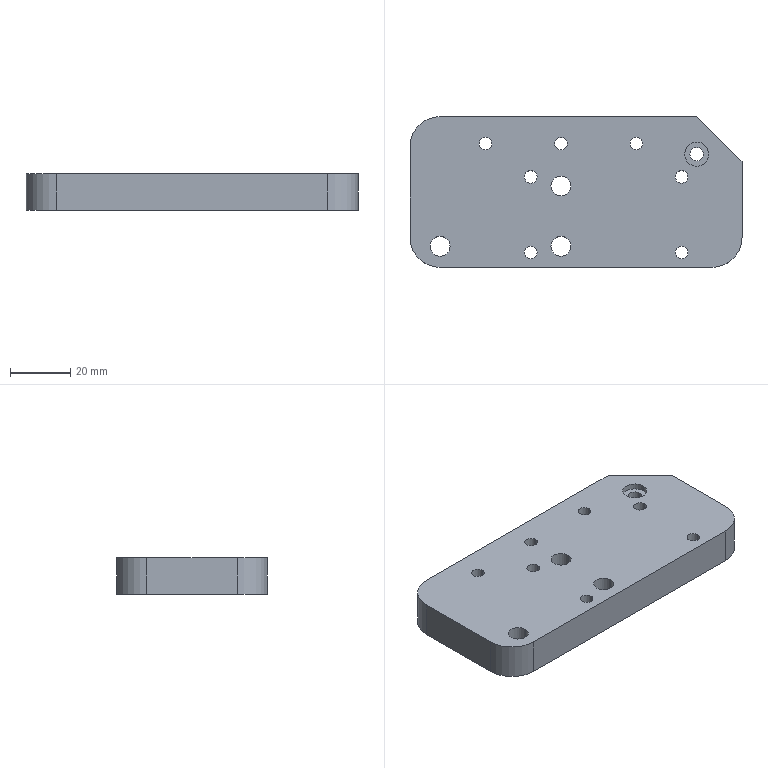Part | STEP file | MT-COMBO-119-S032 | 1 solid | 47 faces | box 110 x 50 x 12 mm | volume 59904 mm3 | cylinder 35 | plane 12 | commonest cylinder face diameters 4.2 x14 6.6 x6 11 x6 8 x4 20 x3 4.5 x2
STEP:
#1=CARTESIAN_POINT('',(-54.5,-43.,6.4));
#2=VERTEX_POINT('',#1);
#3=CARTESIAN_POINT('',(-65.5,-43.,6.4));
#4=VERTEX_POINT('',#3);
#5=CARTESIAN_POINT('',(-60.,-43.,6.4));
#6=DIRECTION('',(0.,0.,-1.));
#7=DIRECTION('',(-1.,0.,0.));
#8=AXIS2_PLACEMENT_3D('',#5,#6,#7);
#9=CIRCLE('',#8,5.5);
#10=EDGE_CURVE('',#2,#4,#9,.T.);
#11=ORIENTED_EDGE('',*,*,#10,.F.);
#12=CARTESIAN_POINT('',(-54.5,-43.,0.));
#13=VERTEX_POINT('',#12);
#14=CARTESIAN_POINT('',(-54.5,-43.,0.));
#15=DIRECTION('',(0.,0.,-1.));
#16=VECTOR('',#15,1000.);
#17=LINE('',#14,#16);
#18=EDGE_CURVE('',#2,#13,#17,.T.);
#19=ORIENTED_EDGE('',*,*,#18,.T.);
#20=CARTESIAN_POINT('',(-65.5,-43.,0.));
#21=VERTEX_POINT('',#20);
#22=CARTESIAN_POINT('',(-60.,-43.,0.));
#23=DIRECTION('',(0.,0.,-1.));
#24=DIRECTION('',(-1.,0.,0.));
#25=AXIS2_PLACEMENT_3D('',#22,#23,#24);
#26=CIRCLE('',#25,5.5);
#27=EDGE_CURVE('',#13,#21,#26,.T.);
#28=ORIENTED_EDGE('',*,*,#27,.T.);
#29=CARTESIAN_POINT('',(-65.5,-43.,0.));
#30=DIRECTION('',(0.,0.,-1.));
#31=VECTOR('',#30,1000.);
#32=LINE('',#29,#31);
#33=EDGE_CURVE('',#4,#21,#32,.T.);
#34=ORIENTED_EDGE('',*,*,#33,.F.);
#35=EDGE_LOOP('',(#11,#19,#28,#34));
#36=FACE_OUTER_BOUND('',#35,.T.);
#37=CARTESIAN_POINT('',(-60.,-43.,0.));
#38=DIRECTION('',(0.,0.,-1.));
#39=DIRECTION('',(-1.,0.,0.));
#40=AXIS2_PLACEMENT_3D('',#37,#38,#39);
#41=CYLINDRICAL_SURFACE('',#40,5.5);
#42=ADVANCED_FACE('',(#36),#41,.F.);
#43=CARTESIAN_POINT('',(-56.7,-43.,12.));
#44=VERTEX_POINT('',#43);
#45=CARTESIAN_POINT('',(-63.3,-43.,12.));
#46=VERTEX_POINT('',#45);
#47=CARTESIAN_POINT('',(-60.,-43.,12.));
#48=DIRECTION('',(0.,0.,-1.));
#49=DIRECTION('',(-1.,0.,0.));
#50=AXIS2_PLACEMENT_3D('',#47,#48,#49);
#51=CIRCLE('',#50,3.3);
#52=EDGE_CURVE('',#44,#46,#51,.T.);
#53=ORIENTED_EDGE('',*,*,#52,.F.);
#54=CARTESIAN_POINT('',(-56.7,-43.,6.4));
#55=VERTEX_POINT('',#54);
#56=CARTESIAN_POINT('',(-56.7,-43.,0.));
#57=DIRECTION('',(0.,0.,-1.));
#58=VECTOR('',#57,1000.);
#59=LINE('',#56,#58);
#60=EDGE_CURVE('',#44,#55,#59,.T.);
#61=ORIENTED_EDGE('',*,*,#60,.T.);
#62=CARTESIAN_POINT('',(-63.3,-43.,6.4));
#63=VERTEX_POINT('',#62);
#64=CARTESIAN_POINT('',(-60.,-43.,6.4));
#65=DIRECTION('',(0.,0.,-1.));
#66=DIRECTION('',(-1.,0.,0.));
#67=AXIS2_PLACEMENT_3D('',#64,#65,#66);
#68=CIRCLE('',#67,3.3);
#69=EDGE_CURVE('',#55,#63,#68,.T.);
#70=ORIENTED_EDGE('',*,*,#69,.T.);
#71=CARTESIAN_POINT('',(-63.3,-43.,0.));
#72=DIRECTION('',(0.,0.,-1.));
#73=VECTOR('',#72,1000.);
#74=LINE('',#71,#73);
#75=EDGE_CURVE('',#46,#63,#74,.T.);
#76=ORIENTED_EDGE('',*,*,#75,.F.);
#77=EDGE_LOOP('',(#53,#61,#70,#76));
#78=FACE_OUTER_BOUND('',#77,.T.);
#79=CARTESIAN_POINT('',(-60.,-43.,0.));
#80=DIRECTION('',(0.,0.,-1.));
#81=DIRECTION('',(-1.,0.,0.));
#82=AXIS2_PLACEMENT_3D('',#79,#80,#81);
#83=CYLINDRICAL_SURFACE('',#82,3.3);
#84=ADVANCED_FACE('',(#78),#83,.F.);
#85=CARTESIAN_POINT('',(-94.5,-43.,6.4));
#86=VERTEX_POINT('',#85);
#87=CARTESIAN_POINT('',(-105.5,-43.,6.4));
#88=VERTEX_POINT('',#87);
#89=CARTESIAN_POINT('',(-100.,-43.,6.4));
#90=DIRECTION('',(0.,0.,-1.));
#91=DIRECTION('',(-1.,0.,0.));
#92=AXIS2_PLACEMENT_3D('',#89,#90,#91);
#93=CIRCLE('',#92,5.5);
#94=EDGE_CURVE('',#86,#88,#93,.T.);
#95=ORIENTED_EDGE('',*,*,#94,.F.);
#96=CARTESIAN_POINT('',(-94.5,-43.,0.));
#97=VERTEX_POINT('',#96);
#98=CARTESIAN_POINT('',(-94.5,-43.,0.));
#99=DIRECTION('',(0.,0.,-1.));
#100=VECTOR('',#99,1000.);
#101=LINE('',#98,#100);
#102=EDGE_CURVE('',#86,#97,#101,.T.);
#103=ORIENTED_EDGE('',*,*,#102,.T.);
#104=CARTESIAN_POINT('',(-105.5,-43.,0.));
#105=VERTEX_POINT('',#104);
#106=CARTESIAN_POINT('',(-100.,-43.,0.));
#107=DIRECTION('',(0.,0.,-1.));
#108=DIRECTION('',(-1.,0.,0.));
#109=AXIS2_PLACEMENT_3D('',#106,#107,#108);
#110=CIRCLE('',#109,5.5);
#111=EDGE_CURVE('',#97,#105,#110,.T.);
#112=ORIENTED_EDGE('',*,*,#111,.T.);
#113=CARTESIAN_POINT('',(-105.5,-43.,0.));
#114=DIRECTION('',(0.,0.,-1.));
#115=VECTOR('',#114,1000.);
#116=LINE('',#113,#115);
#117=EDGE_CURVE('',#88,#105,#116,.T.);
#118=ORIENTED_EDGE('',*,*,#117,.F.);
#119=EDGE_LOOP('',(#95,#103,#112,#118));
#120=FACE_OUTER_BOUND('',#119,.T.);
#121=CARTESIAN_POINT('',(-100.,-43.,0.));
#122=DIRECTION('',(0.,0.,-1.));
#123=DIRECTION('',(-1.,0.,0.));
#124=AXIS2_PLACEMENT_3D('',#121,#122,#123);
#125=CYLINDRICAL_SURFACE('',#124,5.5);
#126=ADVANCED_FACE('',(#120),#125,.F.);
#127=CARTESIAN_POINT('',(-96.7,-43.,12.));
#128=VERTEX_POINT('',#127);
#129=CARTESIAN_POINT('',(-103.3,-43.,12.));
#130=VERTEX_POINT('',#129);
#131=CARTESIAN_POINT('',(-100.,-43.,12.));
#132=DIRECTION('',(0.,0.,-1.));
#133=DIRECTION('',(-1.,0.,0.));
#134=AXIS2_PLACEMENT_3D('',#131,#132,#133);
#135=CIRCLE('',#134,3.3);
#136=EDGE_CURVE('',#128,#130,#135,.T.);
#137=ORIENTED_EDGE('',*,*,#136,.F.);
#138=CARTESIAN_POINT('',(-96.7,-43.,6.4));
#139=VERTEX_POINT('',#138);
#140=CARTESIAN_POINT('',(-96.7,-43.,0.));
#141=DIRECTION('',(0.,0.,-1.));
#142=VECTOR('',#141,1000.);
#143=LINE('',#140,#142);
#144=EDGE_CURVE('',#128,#139,#143,.T.);
#145=ORIENTED_EDGE('',*,*,#144,.T.);
#146=CARTESIAN_POINT('',(-103.3,-43.,6.4));
#147=VERTEX_POINT('',#146);
#148=CARTESIAN_POINT('',(-100.,-43.,6.4));
#149=DIRECTION('',(0.,0.,-1.));
#150=DIRECTION('',(-1.,0.,0.));
#151=AXIS2_PLACEMENT_3D('',#148,#149,#150);
#152=CIRCLE('',#151,3.3);
#153=EDGE_CURVE('',#139,#147,#152,.T.);
#154=ORIENTED_EDGE('',*,*,#153,.T.);
#155=CARTESIAN_POINT('',(-103.3,-43.,0.));
#156=DIRECTION('',(0.,0.,-1.));
#157=VECTOR('',#156,1000.);
#158=LINE('',#155,#157);
#159=EDGE_CURVE('',#130,#147,#158,.T.);
#160=ORIENTED_EDGE('',*,*,#159,.F.);
#161=EDGE_LOOP('',(#137,#145,#154,#160));
#162=FACE_OUTER_BOUND('',#161,.T.);
#163=CARTESIAN_POINT('',(-100.,-43.,0.));
#164=DIRECTION('',(0.,0.,-1.));
#165=DIRECTION('',(-1.,0.,0.));
#166=AXIS2_PLACEMENT_3D('',#163,#164,#165);
#167=CYLINDRICAL_SURFACE('',#166,3.3);
#168=ADVANCED_FACE('',(#162),#167,.F.);
#169=CARTESIAN_POINT('',(-54.5,-23.,6.4));
#170=VERTEX_POINT('',#169);
#171=CARTESIAN_POINT('',(-65.5,-23.,6.4));
#172=VERTEX_POINT('',#171);
#173=CARTESIAN_POINT('',(-60.,-23.,6.4));
#174=DIRECTION('',(0.,0.,-1.));
#175=DIRECTION('',(-1.,0.,0.));
#176=AXIS2_PLACEMENT_3D('',#173,#174,#175);
#177=CIRCLE('',#176,5.5);
#178=EDGE_CURVE('',#170,#172,#177,.T.);
#179=ORIENTED_EDGE('',*,*,#178,.F.);
#180=CARTESIAN_POINT('',(-54.5,-23.,0.));
#181=VERTEX_POINT('',#180);
#182=CARTESIAN_POINT('',(-54.5,-23.,0.));
#183=DIRECTION('',(0.,0.,-1.));
#184=VECTOR('',#183,1000.);
#185=LINE('',#182,#184);
#186=EDGE_CURVE('',#170,#181,#185,.T.);
#187=ORIENTED_EDGE('',*,*,#186,.T.);
#188=CARTESIAN_POINT('',(-65.5,-23.,0.));
#189=VERTEX_POINT('',#188);
#190=CARTESIAN_POINT('',(-60.,-23.,0.));
#191=DIRECTION('',(0.,0.,-1.));
#192=DIRECTION('',(-1.,0.,0.));
#193=AXIS2_PLACEMENT_3D('',#190,#191,#192);
#194=CIRCLE('',#193,5.5);
#195=EDGE_CURVE('',#181,#189,#194,.T.);
#196=ORIENTED_EDGE('',*,*,#195,.T.);
#197=CARTESIAN_POINT('',(-65.5,-23.,0.));
#198=DIRECTION('',(0.,0.,-1.));
#199=VECTOR('',#198,1000.);
#200=LINE('',#197,#199);
#201=EDGE_CURVE('',#172,#189,#200,.T.);
#202=ORIENTED_EDGE('',*,*,#201,.F.);
#203=EDGE_LOOP('',(#179,#187,#196,#202));
#204=FACE_OUTER_BOUND('',#203,.T.);
#205=CARTESIAN_POINT('',(-60.,-23.,0.));
#206=DIRECTION('',(0.,0.,-1.));
#207=DIRECTION('',(-1.,0.,0.));
#208=AXIS2_PLACEMENT_3D('',#205,#206,#207);
#209=CYLINDRICAL_SURFACE('',#208,5.5);
#210=ADVANCED_FACE('',(#204),#209,.F.);
#211=CARTESIAN_POINT('',(-56.7,-23.,12.));
#212=VERTEX_POINT('',#211);
#213=CARTESIAN_POINT('',(-63.3,-23.,12.));
#214=VERTEX_POINT('',#213);
#215=CARTESIAN_POINT('',(-60.,-23.,12.));
#216=DIRECTION('',(0.,0.,-1.));
#217=DIRECTION('',(-1.,0.,0.));
#218=AXIS2_PLACEMENT_3D('',#215,#216,#217);
#219=CIRCLE('',#218,3.3);
#220=EDGE_CURVE('',#212,#214,#219,.T.);
#221=ORIENTED_EDGE('',*,*,#220,.F.);
#222=CARTESIAN_POINT('',(-56.7,-23.,6.4));
#223=VERTEX_POINT('',#222);
#224=CARTESIAN_POINT('',(-56.7,-23.,0.));
#225=DIRECTION('',(0.,0.,-1.));
#226=VECTOR('',#225,1000.);
#227=LINE('',#224,#226);
#228=EDGE_CURVE('',#212,#223,#227,.T.);
#229=ORIENTED_EDGE('',*,*,#228,.T.);
#230=CARTESIAN_POINT('',(-63.3,-23.,6.4));
#231=VERTEX_POINT('',#230);
#232=CARTESIAN_POINT('',(-60.,-23.,6.4));
#233=DIRECTION('',(0.,0.,-1.));
#234=DIRECTION('',(-1.,0.,0.));
#235=AXIS2_PLACEMENT_3D('',#232,#233,#234);
#236=CIRCLE('',#235,3.3);
#237=EDGE_CURVE('',#223,#231,#236,.T.);
#238=ORIENTED_EDGE('',*,*,#237,.T.);
#239=CARTESIAN_POINT('',(-63.3,-23.,0.));
#240=DIRECTION('',(0.,0.,-1.));
#241=VECTOR('',#240,1000.);
#242=LINE('',#239,#241);
#243=EDGE_CURVE('',#214,#231,#242,.T.);
#244=ORIENTED_EDGE('',*,*,#243,.F.);
#245=EDGE_LOOP('',(#221,#229,#238,#244));
#246=FACE_OUTER_BOUND('',#245,.T.);
#247=CARTESIAN_POINT('',(-60.,-23.,0.));
#248=DIRECTION('',(0.,0.,-1.));
#249=DIRECTION('',(-1.,0.,0.));
#250=AXIS2_PLACEMENT_3D('',#247,#248,#249);
#251=CYLINDRICAL_SURFACE('',#250,3.3);
#252=ADVANCED_FACE('',(#246),#251,.F.);
#253=CARTESIAN_POINT('',(-32.9,-9.,12.));
#254=VERTEX_POINT('',#253);
#255=CARTESIAN_POINT('',(-37.1,-9.,12.));
#256=VERTEX_POINT('',#255);
#257=CARTESIAN_POINT('',(-35.,-9.,12.));
#258=DIRECTION('',(0.,0.,-1.));
#259=DIRECTION('',(-1.,0.,0.));
#260=AXIS2_PLACEMENT_3D('',#257,#258,#259);
#261=CIRCLE('',#260,2.1);
#262=EDGE_CURVE('',#254,#256,#261,.T.);
#263=ORIENTED_EDGE('',*,*,#262,.F.);
#264=CARTESIAN_POINT('',(-32.9,-9.,0.));
#265=VERTEX_POINT('',#264);
#266=CARTESIAN_POINT('',(-32.9,-9.,0.));
#267=DIRECTION('',(0.,0.,-1.));
#268=VECTOR('',#267,1000.);
#269=LINE('',#266,#268);
#270=EDGE_CURVE('',#254,#265,#269,.T.);
#271=ORIENTED_EDGE('',*,*,#270,.T.);
#272=CARTESIAN_POINT('',(-37.1,-9.,0.));
#273=VERTEX_POINT('',#272);
#274=CARTESIAN_POINT('',(-35.,-9.,0.));
#275=DIRECTION('',(0.,0.,-1.));
#276=DIRECTION('',(-1.,0.,0.));
#277=AXIS2_PLACEMENT_3D('',#274,#275,#276);
#278=CIRCLE('',#277,2.1);
#279=EDGE_CURVE('',#265,#273,#278,.T.);
#280=ORIENTED_EDGE('',*,*,#279,.T.);
#281=CARTESIAN_POINT('',(-37.1,-9.,0.));
#282=DIRECTION('',(0.,0.,-1.));
#283=VECTOR('',#282,1000.);
#284=LINE('',#281,#283);
#285=EDGE_CURVE('',#256,#273,#284,.T.);
#286=ORIENTED_EDGE('',*,*,#285,.F.);
#287=EDGE_LOOP('',(#263,#271,#280,#286));
#288=FACE_OUTER_BOUND('',#287,.T.);
#289=CARTESIAN_POINT('',(-35.,-9.,0.));
#290=DIRECTION('',(0.,0.,-1.));
#291=DIRECTION('',(-1.,0.,0.));
#292=AXIS2_PLACEMENT_3D('',#289,#290,#291);
#293=CYLINDRICAL_SURFACE('',#292,2.1);
#294=ADVANCED_FACE('',(#288),#293,.F.);
#295=CARTESIAN_POINT('',(-57.9,-9.,12.));
#296=VERTEX_POINT('',#295);
#297=CARTESIAN_POINT('',(-62.1,-9.,12.));
#298=VERTEX_POINT('',#297);
#299=CARTESIAN_POINT('',(-60.,-9.,12.));
#300=DIRECTION('',(0.,0.,-1.));
#301=DIRECTION('',(-1.,0.,0.));
#302=AXIS2_PLACEMENT_3D('',#299,#300,#301);
#303=CIRCLE('',#302,2.1);
#304=EDGE_CURVE('',#296,#298,#303,.T.);
#305=ORIENTED_EDGE('',*,*,#304,.F.);
#306=CARTESIAN_POINT('',(-57.9,-9.,0.));
#307=VERTEX_POINT('',#306);
#308=CARTESIAN_POINT('',(-57.9,-9.,0.));
#309=DIRECTION('',(0.,0.,-1.));
#310=VECTOR('',#309,1000.);
#311=LINE('',#308,#310);
#312=EDGE_CURVE('',#296,#307,#311,.T.);
#313=ORIENTED_EDGE('',*,*,#312,.T.);
#314=CARTESIAN_POINT('',(-62.1,-9.,0.));
#315=VERTEX_POINT('',#314);
#316=CARTESIAN_POINT('',(-60.,-9.,0.));
#317=DIRECTION('',(0.,0.,-1.));
#318=DIRECTION('',(-1.,0.,0.));
#319=AXIS2_PLACEMENT_3D('',#316,#317,#318);
#320=CIRCLE('',#319,2.1);
#321=EDGE_CURVE('',#307,#315,#320,.T.);
#322=ORIENTED_EDGE('',*,*,#321,.T.);
#323=CARTESIAN_POINT('',(-62.1,-9.,0.));
#324=DIRECTION('',(0.,0.,-1.));
#325=VECTOR('',#324,1000.);
#326=LINE('',#323,#325);
#327=EDGE_CURVE('',#298,#315,#326,.T.);
#328=ORIENTED_EDGE('',*,*,#327,.F.);
#329=EDGE_LOOP('',(#305,#313,#322,#328));
#330=FACE_OUTER_BOUND('',#329,.T.);
#331=CARTESIAN_POINT('',(-60.,-9.,0.));
#332=DIRECTION('',(0.,0.,-1.));
#333=DIRECTION('',(-1.,0.,0.));
#334=AXIS2_PLACEMENT_3D('',#331,#332,#333);
#335=CYLINDRICAL_SURFACE('',#334,2.1);
#336=ADVANCED_FACE('',(#330),#335,.F.);
#337=CARTESIAN_POINT('',(-82.9,-9.,12.));
#338=VERTEX_POINT('',#337);
#339=CARTESIAN_POINT('',(-87.1,-9.,12.));
#340=VERTEX_POINT('',#339);
#341=CARTESIAN_POINT('',(-85.,-9.,12.));
#342=DIRECTION('',(0.,0.,-1.));
#343=DIRECTION('',(-1.,0.,0.));
#344=AXIS2_PLACEMENT_3D('',#341,#342,#343);
#345=CIRCLE('',#344,2.1);
#346=EDGE_CURVE('',#338,#340,#345,.T.);
#347=ORIENTED_EDGE('',*,*,#346,.F.);
#348=CARTESIAN_POINT('',(-82.9,-9.,0.));
#349=VERTEX_POINT('',#348);
#350=CARTESIAN_POINT('',(-82.9,-9.,0.));
#351=DIRECTION('',(0.,0.,-1.));
#352=VECTOR('',#351,1000.);
#353=LINE('',#350,#352);
#354=EDGE_CURVE('',#338,#349,#353,.T.);
#355=ORIENTED_EDGE('',*,*,#354,.T.);
#356=CARTESIAN_POINT('',(-87.1,-9.,0.));
#357=VERTEX_POINT('',#356);
#358=CARTESIAN_POINT('',(-85.,-9.,0.));
#359=DIRECTION('',(0.,0.,-1.));
#360=DIRECTION('',(-1.,0.,0.));
#361=AXIS2_PLACEMENT_3D('',#358,#359,#360);
#362=CIRCLE('',#361,2.1);
#363=EDGE_CURVE('',#349,#357,#362,.T.);
#364=ORIENTED_EDGE('',*,*,#363,.T.);
#365=CARTESIAN_POINT('',(-87.1,-9.,0.));
#366=DIRECTION('',(0.,0.,-1.));
#367=VECTOR('',#366,1000.);
#368=LINE('',#365,#367);
#369=EDGE_CURVE('',#340,#357,#368,.T.);
#370=ORIENTED_EDGE('',*,*,#369,.F.);
#371=EDGE_LOOP('',(#347,#355,#364,#370));
#372=FACE_OUTER_BOUND('',#371,.T.);
#373=CARTESIAN_POINT('',(-85.,-9.,0.));
#374=DIRECTION('',(0.,0.,-1.));
#375=DIRECTION('',(-1.,0.,0.));
#376=AXIS2_PLACEMENT_3D('',#373,#374,#375);
#377=CYLINDRICAL_SURFACE('',#376,2.1);
#378=ADVANCED_FACE('',(#372),#377,.F.);
#379=CARTESIAN_POINT('',(-67.9,-20.,12.));
#380=VERTEX_POINT('',#379);
#381=CARTESIAN_POINT('',(-72.1,-20.,12.));
#382=VERTEX_POINT('',#381);
#383=CARTESIAN_POINT('',(-70.,-20.,12.));
#384=DIRECTION('',(0.,0.,-1.));
#385=DIRECTION('',(-1.,0.,0.));
#386=AXIS2_PLACEMENT_3D('',#383,#384,#385);
#387=CIRCLE('',#386,2.1);
#388=EDGE_CURVE('',#380,#382,#387,.T.);
#389=ORIENTED_EDGE('',*,*,#388,.F.);
#390=CARTESIAN_POINT('',(-67.9,-20.,0.));
#391=VERTEX_POINT('',#390);
#392=CARTESIAN_POINT('',(-67.9,-20.,0.));
#393=DIRECTION('',(0.,0.,-1.));
#394=VECTOR('',#393,1000.);
#395=LINE('',#392,#394);
#396=EDGE_CURVE('',#380,#391,#395,.T.);
#397=ORIENTED_EDGE('',*,*,#396,.T.);
#398=CARTESIAN_POINT('',(-72.1,-20.,0.));
#399=VERTEX_POINT('',#398);
#400=CARTESIAN_POINT('',(-70.,-20.,0.));
#401=DIRECTION('',(0.,0.,-1.));
#402=DIRECTION('',(-1.,0.,0.));
#403=AXIS2_PLACEMENT_3D('',#400,#401,#402);
#404=CIRCLE('',#403,2.1);
#405=EDGE_CURVE('',#391,#399,#404,.T.);
#406=ORIENTED_EDGE('',*,*,#405,.T.);
#407=CARTESIAN_POINT('',(-72.1,-20.,0.));
#408=DIRECTION('',(0.,0.,-1.));
#409=VECTOR('',#408,1000.);
#410=LINE('',#407,#409);
#411=EDGE_CURVE('',#382,#399,#410,.T.);
#412=ORIENTED_EDGE('',*,*,#411,.F.);
#413=EDGE_LOOP('',(#389,#397,#406,#412));
#414=FACE_OUTER_BOUND('',#413,.T.);
#415=CARTESIAN_POINT('',(-70.,-20.,0.));
#416=DIRECTION('',(0.,0.,-1.));
#417=DIRECTION('',(-1.,0.,0.));
#418=AXIS2_PLACEMENT_3D('',#415,#416,#417);
#419=CYLINDRICAL_SURFACE('',#418,2.1);
#420=ADVANCED_FACE('',(#414),#419,.F.);
#421=CARTESIAN_POINT('',(-67.9,-45.,12.));
#422=VERTEX_POINT('',#421);
#423=CARTESIAN_POINT('',(-72.1,-45.,12.));
#424=VERTEX_POINT('',#423);
#425=CARTESIAN_POINT('',(-70.,-45.,12.));
#426=DIRECTION('',(0.,0.,-1.));
#427=DIRECTION('',(-1.,0.,0.));
#428=AXIS2_PLACEMENT_3D('',#425,#426,#427);
#429=CIRCLE('',#428,2.1);
#430=EDGE_CURVE('',#422,#424,#429,.T.);
#431=ORIENTED_EDGE('',*,*,#430,.F.);
#432=CARTESIAN_POINT('',(-67.9,-45.,0.));
#433=VERTEX_POINT('',#432);
#434=CARTESIAN_POINT('',(-67.9,-45.,0.));
#435=DIRECTION('',(0.,0.,-1.));
#436=VECTOR('',#435,1000.);
#437=LINE('',#434,#436);
#438=EDGE_CURVE('',#422,#433,#437,.T.);
#439=ORIENTED_EDGE('',*,*,#438,.T.);
#440=CARTESIAN_POINT('',(-72.1,-45.,0.));
#441=VERTEX_POINT('',#440);
#442=CARTESIAN_POINT('',(-70.,-45.,0.));
#443=DIRECTION('',(0.,0.,-1.));
#444=DIRECTION('',(-1.,0.,0.));
#445=AXIS2_PLACEMENT_3D('',#442,#443,#444);
#446=CIRCLE('',#445,2.1);
#447=EDGE_CURVE('',#433,#441,#446,.T.);
#448=ORIENTED_EDGE('',*,*,#447,.T.);
#449=CARTESIAN_POINT('',(-72.1,-45.,0.));
#450=DIRECTION('',(0.,0.,-1.));
#451=VECTOR('',#450,1000.);
#452=LINE('',#449,#451);
#453=EDGE_CURVE('',#424,#441,#452,.T.);
#454=ORIENTED_EDGE('',*,*,#453,.F.);
#455=EDGE_LOOP('',(#431,#439,#448,#454));
#456=FACE_OUTER_BOUND('',#455,.T.);
#457=CARTESIAN_POINT('',(-70.,-45.,0.));
#458=DIRECTION('',(0.,0.,-1.));
#459=DIRECTION('',(-1.,0.,0.));
#460=AXIS2_PLACEMENT_3D('',#457,#458,#459);
#461=CYLINDRICAL_SURFACE('',#460,2.1);
#462=ADVANCED_FACE('',(#456),#461,.F.);
#463=CARTESIAN_POINT('',(-17.9,-45.,12.));
#464=VERTEX_POINT('',#463);
#465=CARTESIAN_POINT('',(-22.1,-45.,12.));
#466=VERTEX_POINT('',#465);
#467=CARTESIAN_POINT('',(-20.,-45.,12.));
#468=DIRECTION('',(0.,0.,-1.));
#469=DIRECTION('',(-1.,0.,0.));
#470=AXIS2_PLACEMENT_3D('',#467,#468,#469);
#471=CIRCLE('',#470,2.1);
#472=EDGE_CURVE('',#464,#466,#471,.T.);
#473=ORIENTED_EDGE('',*,*,#472,.F.);
#474=CARTESIAN_POINT('',(-17.9,-45.,0.));
#475=VERTEX_POINT('',#474);
#476=CARTESIAN_POINT('',(-17.9,-45.,0.));
#477=DIRECTION('',(0.,0.,-1.));
#478=VECTOR('',#477,1000.);
#479=LINE('',#476,#478);
#480=EDGE_CURVE('',#464,#475,#479,.T.);
#481=ORIENTED_EDGE('',*,*,#480,.T.);
#482=CARTESIAN_POINT('',(-22.1,-45.,0.));
#483=VERTEX_POINT('',#482);
#484=CARTESIAN_POINT('',(-20.,-45.,0.));
#485=DIRECTION('',(0.,0.,-1.));
#486=DIRECTION('',(-1.,0.,0.));
#487=AXIS2_PLACEMENT_3D('',#484,#485,#486);
#488=CIRCLE('',#487,2.1);
#489=EDGE_CURVE('',#475,#483,#488,.T.);
#490=ORIENTED_EDGE('',*,*,#489,.T.);
#491=CARTESIAN_POINT('',(-22.1,-45.,0.));
#492=DIRECTION('',(0.,0.,-1.));
#493=VECTOR('',#492,1000.);
#494=LINE('',#491,#493);
#495=EDGE_CURVE('',#466,#483,#494,.T.);
#496=ORIENTED_EDGE('',*,*,#495,.F.);
#497=EDGE_LOOP('',(#473,#481,#490,#496));
#498=FACE_OUTER_BOUND('',#497,.T.);
#499=CARTESIAN_POINT('',(-20.,-45.,0.));
#500=DIRECTION('',(0.,0.,-1.));
#501=DIRECTION('',(-1.,0.,0.));
#502=AXIS2_PLACEMENT_3D('',#499,#500,#501);
#503=CYLINDRICAL_SURFACE('',#502,2.1);
#504=ADVANCED_FACE('',(#498),#503,.F.);
#505=CARTESIAN_POINT('',(-17.9,-20.,12.));
#506=VERTEX_POINT('',#505);
#507=CARTESIAN_POINT('',(-22.1,-20.,12.));
#508=VERTEX_POINT('',#507);
#509=CARTESIAN_POINT('',(-20.,-20.,12.));
#510=DIRECTION('',(0.,0.,-1.));
#511=DIRECTION('',(-1.,0.,0.));
#512=AXIS2_PLACEMENT_3D('',#509,#510,#511);
#513=CIRCLE('',#512,2.1);
#514=EDGE_CURVE('',#506,#508,#513,.T.);
#515=ORIENTED_EDGE('',*,*,#514,.F.);
#516=CARTESIAN_POINT('',(-17.9,-20.,0.));
#517=VERTEX_POINT('',#516);
#518=CARTESIAN_POINT('',(-17.9,-20.,0.));
#519=DIRECTION('',(0.,0.,-1.));
#520=VECTOR('',#519,1000.);
#521=LINE('',#518,#520);
#522=EDGE_CURVE('',#506,#517,#521,.T.);
#523=ORIENTED_EDGE('',*,*,#522,.T.);
#524=CARTESIAN_POINT('',(-22.1,-20.,0.));
#525=VERTEX_POINT('',#524);
#526=CARTESIAN_POINT('',(-20.,-20.,0.));
#527=DIRECTION('',(0.,0.,-1.));
#528=DIRECTION('',(-1.,0.,0.));
#529=AXIS2_PLACEMENT_3D('',#526,#527,#528);
#530=CIRCLE('',#529,2.1);
#531=EDGE_CURVE('',#517,#525,#530,.T.);
#532=ORIENTED_EDGE('',*,*,#531,.T.);
#533=CARTESIAN_POINT('',(-22.1,-20.,0.));
#534=DIRECTION('',(0.,0.,-1.));
#535=VECTOR('',#534,1000.);
#536=LINE('',#533,#535);
#537=EDGE_CURVE('',#508,#525,#536,.T.);
#538=ORIENTED_EDGE('',*,*,#537,.F.);
#539=EDGE_LOOP('',(#515,#523,#532,#538));
#540=FACE_OUTER_BOUND('',#539,.T.);
#541=CARTESIAN_POINT('',(-20.,-20.,0.));
#542=DIRECTION('',(0.,0.,-1.));
#543=DIRECTION('',(-1.,0.,0.));
#544=AXIS2_PLACEMENT_3D('',#541,#542,#543);
#545=CYLINDRICAL_SURFACE('',#544,2.1);
#546=ADVANCED_FACE('',(#540),#545,.F.);
#547=CARTESIAN_POINT('',(-19.,-12.5,10.));
#548=VERTEX_POINT('',#547);
#549=CARTESIAN_POINT('',(-11.,-12.5,10.));
#550=VERTEX_POINT('',#549);
#551=CARTESIAN_POINT('',(-15.,-12.5,10.));
#552=DIRECTION('',(0.,0.,1.));
#553=DIRECTION('',(1.,0.,0.));
#554=AXIS2_PLACEMENT_3D('',#551,#552,#553);
#555=CIRCLE('',#554,4.);
#556=EDGE_CURVE('',#548,#550,#555,.T.);
#557=ORIENTED_EDGE('',*,*,#556,.F.);
#558=CARTESIAN_POINT('',(-19.,-12.5,12.));
#559=VERTEX_POINT('',#558);
#560=CARTESIAN_POINT('',(-19.,-12.5,12.));
#561=DIRECTION('',(0.,0.,1.));
#562=VECTOR('',#561,1000.);
#563=LINE('',#560,#562);
#564=EDGE_CURVE('',#548,#559,#563,.T.);
#565=ORIENTED_EDGE('',*,*,#564,.T.);
#566=CARTESIAN_POINT('',(-11.,-12.5,12.));
#567=VERTEX_POINT('',#566);
#568=CARTESIAN_POINT('',(-15.,-12.5,12.));
#569=DIRECTION('',(0.,0.,1.));
#570=DIRECTION('',(1.,0.,0.));
#571=AXIS2_PLACEMENT_3D('',#568,#569,#570);
#572=CIRCLE('',#571,4.);
#573=EDGE_CURVE('',#559,#567,#572,.T.);
#574=ORIENTED_EDGE('',*,*,#573,.T.);
#575=CARTESIAN_POINT('',(-11.,-12.5,12.));
#576=DIRECTION('',(0.,0.,1.));
#577=VECTOR('',#576,1000.);
#578=LINE('',#575,#577);
#579=EDGE_CURVE('',#550,#567,#578,.T.);
#580=ORIENTED_EDGE('',*,*,#579,.F.);
#581=EDGE_LOOP('',(#557,#565,#574,#580));
#582=FACE_OUTER_BOUND('',#581,.T.);
#583=CARTESIAN_POINT('',(-15.,-12.5,12.));
#584=DIRECTION('',(0.,0.,1.));
#585=DIRECTION('',(1.,0.,0.));
#586=AXIS2_PLACEMENT_3D('',#583,#584,#585);
#587=CYLINDRICAL_SURFACE('',#586,4.);
#588=ADVANCED_FACE('',(#582),#587,.F.);
#589=CARTESIAN_POINT('',(-11.,-12.5,4.4));
#590=VERTEX_POINT('',#589);
#591=CARTESIAN_POINT('',(-19.,-12.5,4.4));
#592=VERTEX_POINT('',#591);
#593=CARTESIAN_POINT('',(-15.,-12.5,4.4));
#594=DIRECTION('',(0.,0.,-1.));
#595=DIRECTION('',(-1.,0.,0.));
#596=AXIS2_PLACEMENT_3D('',#593,#594,#595);
#597=CIRCLE('',#596,4.);
#598=EDGE_CURVE('',#590,#592,#597,.T.);
#599=ORIENTED_EDGE('',*,*,#598,.F.);
#600=CARTESIAN_POINT('',(-11.,-12.5,0.));
#601=VERTEX_POINT('',#600);
#602=CARTESIAN_POINT('',(-11.,-12.5,0.));
#603=DIRECTION('',(0.,0.,-1.));
#604=VECTOR('',#603,1000.);
#605=LINE('',#602,#604);
#606=EDGE_CURVE('',#590,#601,#605,.T.);
#607=ORIENTED_EDGE('',*,*,#606,.T.);
#608=CARTESIAN_POINT('',(-19.,-12.5,0.));
#609=VERTEX_POINT('',#608);
#610=CARTESIAN_POINT('',(-15.,-12.5,0.));
#611=DIRECTION('',(0.,0.,-1.));
#612=DIRECTION('',(-1.,0.,0.));
#613=AXIS2_PLACEMENT_3D('',#610,#611,#612);
#614=CIRCLE('',#613,4.);
#615=EDGE_CURVE('',#601,#609,#614,.T.);
#616=ORIENTED_EDGE('',*,*,#615,.T.);
#617=CARTESIAN_POINT('',(-19.,-12.5,0.));
#618=DIRECTION('',(0.,0.,-1.));
#619=VECTOR('',#618,1000.);
#620=LINE('',#617,#619);
#621=EDGE_CURVE('',#592,#609,#620,.T.);
#622=ORIENTED_EDGE('',*,*,#621,.F.);
#623=EDGE_LOOP('',(#599,#607,#616,#622));
#624=FACE_OUTER_BOUND('',#623,.T.);
#625=CARTESIAN_POINT('',(-15.,-12.5,0.));
#626=DIRECTION('',(0.,0.,-1.));
#627=DIRECTION('',(-1.,0.,0.));
#628=AXIS2_PLACEMENT_3D('',#625,#626,#627);
#629=CYLINDRICAL_SURFACE('',#628,4.);
#630=ADVANCED_FACE('',(#624),#629,.F.);
#631=CARTESIAN_POINT('',(-17.25,-12.5,10.));
#632=VERTEX_POINT('',#631);
#633=CARTESIAN_POINT('',(-12.75,-12.5,10.));
#634=VERTEX_POINT('',#633);
#635=CARTESIAN_POINT('',(-15.,-12.5,10.));
#636=DIRECTION('',(0.,0.,1.));
#637=DIRECTION('',(-1.,0.,0.));
#638=AXIS2_PLACEMENT_3D('',#635,#636,#637);
#639=CIRCLE('',#638,2.25);
#640=EDGE_CURVE('',#632,#634,#639,.T.);
#641=ORIENTED_EDGE('',*,*,#640,.T.);
#642=CARTESIAN_POINT('',(-12.75,-12.5,4.4));
#643=VERTEX_POINT('',#642);
#644=CARTESIAN_POINT('',(-12.75,-12.5,0.));
#645=DIRECTION('',(0.,0.,-1.));
#646=VECTOR('',#645,1000.);
#647=LINE('',#644,#646);
#648=EDGE_CURVE('',#634,#643,#647,.T.);
#649=ORIENTED_EDGE('',*,*,#648,.T.);
#650=CARTESIAN_POINT('',(-17.25,-12.5,4.4));
#651=VERTEX_POINT('',#650);
#652=CARTESIAN_POINT('',(-15.,-12.5,4.4));
#653=DIRECTION('',(0.,0.,-1.));
#654=DIRECTION('',(-1.,0.,0.));
#655=AXIS2_PLACEMENT_3D('',#652,#653,#654);
#656=CIRCLE('',#655,2.25);
#657=EDGE_CURVE('',#643,#651,#656,.T.);
#658=ORIENTED_EDGE('',*,*,#657,.T.);
#659=CARTESIAN_POINT('',(-17.25,-12.5,0.));
#660=DIRECTION('',(0.,0.,-1.));
#661=VECTOR('',#660,1000.);
#662=LINE('',#659,#661);
#663=EDGE_CURVE('',#632,#651,#662,.T.);
#664=ORIENTED_EDGE('',*,*,#663,.F.);
#665=EDGE_LOOP('',(#641,#649,#658,#664));
#666=FACE_OUTER_BOUND('',#665,.T.);
#667=CARTESIAN_POINT('',(-15.,-12.5,0.));
#668=DIRECTION('',(0.,0.,-1.));
#669=DIRECTION('',(-1.,0.,0.));
#670=AXIS2_PLACEMENT_3D('',#667,#668,#669);
#671=CYLINDRICAL_SURFACE('',#670,2.25);
#672=ADVANCED_FACE('',(#666),#671,.F.);
#673=CARTESIAN_POINT('',(-60.,-43.,0.));
#674=DIRECTION('',(0.,0.,-1.));
#675=DIRECTION('',(-1.,0.,0.));
#676=AXIS2_PLACEMENT_3D('',#673,#674,#675);
#677=CIRCLE('',#676,5.5);
#678=EDGE_CURVE('',#21,#13,#677,.T.);
#679=ORIENTED_EDGE('',*,*,#678,.F.);
#680=ORIENTED_EDGE('',*,*,#27,.F.);
#681=EDGE_LOOP('',(#679,#680));
#682=FACE_BOUND('',#681,.T.);
#683=CARTESIAN_POINT('',(-100.,-43.,0.));
#684=DIRECTION('',(0.,0.,-1.));
#685=DIRECTION('',(-1.,0.,0.));
#686=AXIS2_PLACEMENT_3D('',#683,#684,#685);
#687=CIRCLE('',#686,5.5);
#688=EDGE_CURVE('',#105,#97,#687,.T.);
#689=ORIENTED_EDGE('',*,*,#688,.F.);
#690=ORIENTED_EDGE('',*,*,#111,.F.);
#691=EDGE_LOOP('',(#689,#690));
#692=FACE_BOUND('',#691,.T.);
#693=CARTESIAN_POINT('',(-60.,-23.,0.));
#694=DIRECTION('',(0.,0.,-1.));
#695=DIRECTION('',(-1.,0.,0.));
#696=AXIS2_PLACEMENT_3D('',#693,#694,#695);
#697=CIRCLE('',#696,5.5);
#698=EDGE_CURVE('',#189,#181,#697,.T.);
#699=ORIENTED_EDGE('',*,*,#698,.F.);
#700=ORIENTED_EDGE('',*,*,#195,.F.);
#701=EDGE_LOOP('',(#699,#700));
#702=FACE_BOUND('',#701,.T.);
#703=CARTESIAN_POINT('',(-35.,-9.,0.));
#704=DIRECTION('',(0.,0.,-1.));
#705=DIRECTION('',(-1.,0.,0.));
#706=AXIS2_PLACEMENT_3D('',#703,#704,#705);
#707=CIRCLE('',#706,2.1);
#708=EDGE_CURVE('',#273,#265,#707,.T.);
#709=ORIENTED_EDGE('',*,*,#708,.F.);
#710=ORIENTED_EDGE('',*,*,#279,.F.);
#711=EDGE_LOOP('',(#709,#710));
#712=FACE_BOUND('',#711,.T.);
#713=CARTESIAN_POINT('',(-60.,-9.,0.));
#714=DIRECTION('',(0.,0.,-1.));
#715=DIRECTION('',(-1.,0.,0.));
#716=AXIS2_PLACEMENT_3D('',#713,#714,#715);
#717=CIRCLE('',#716,2.1);
#718=EDGE_CURVE('',#315,#307,#717,.T.);
#719=ORIENTED_EDGE('',*,*,#718,.F.);
#720=ORIENTED_EDGE('',*,*,#321,.F.);
#721=EDGE_LOOP('',(#719,#720));
#722=FACE_BOUND('',#721,.T.);
#723=CARTESIAN_POINT('',(-85.,-9.,0.));
#724=DIRECTION('',(0.,0.,-1.));
#725=DIRECTION('',(-1.,0.,0.));
#726=AXIS2_PLACEMENT_3D('',#723,#724,#725);
#727=CIRCLE('',#726,2.1);
#728=EDGE_CURVE('',#357,#349,#727,.T.);
#729=ORIENTED_EDGE('',*,*,#728,.F.);
#730=ORIENTED_EDGE('',*,*,#363,.F.);
#731=EDGE_LOOP('',(#729,#730));
#732=FACE_BOUND('',#731,.T.);
#733=CARTESIAN_POINT('',(-70.,-20.,0.));
#734=DIRECTION('',(0.,0.,-1.));
#735=DIRECTION('',(-1.,0.,0.));
#736=AXIS2_PLACEMENT_3D('',#733,#734,#735);
#737=CIRCLE('',#736,2.1);
#738=EDGE_CURVE('',#399,#391,#737,.T.);
#739=ORIENTED_EDGE('',*,*,#738,.F.);
#740=ORIENTED_EDGE('',*,*,#405,.F.);
#741=EDGE_LOOP('',(#739,#740));
#742=FACE_BOUND('',#741,.T.);
#743=CARTESIAN_POINT('',(-70.,-45.,0.));
#744=DIRECTION('',(0.,0.,-1.));
#745=DIRECTION('',(-1.,0.,0.));
#746=AXIS2_PLACEMENT_3D('',#743,#744,#745);
#747=CIRCLE('',#746,2.1);
#748=EDGE_CURVE('',#441,#433,#747,.T.);
#749=ORIENTED_EDGE('',*,*,#748,.F.);
#750=ORIENTED_EDGE('',*,*,#447,.F.);
#751=EDGE_LOOP('',(#749,#750));
#752=FACE_BOUND('',#751,.T.);
#753=CARTESIAN_POINT('',(-20.,-45.,0.));
#754=DIRECTION('',(0.,0.,-1.));
#755=DIRECTION('',(-1.,0.,0.));
#756=AXIS2_PLACEMENT_3D('',#753,#754,#755);
#757=CIRCLE('',#756,2.1);
#758=EDGE_CURVE('',#483,#475,#757,.T.);
#759=ORIENTED_EDGE('',*,*,#758,.F.);
#760=ORIENTED_EDGE('',*,*,#489,.F.);
#761=EDGE_LOOP('',(#759,#760));
#762=FACE_BOUND('',#761,.T.);
#763=CARTESIAN_POINT('',(-20.,-20.,0.));
#764=DIRECTION('',(0.,0.,-1.));
#765=DIRECTION('',(-1.,0.,0.));
#766=AXIS2_PLACEMENT_3D('',#763,#764,#765);
#767=CIRCLE('',#766,2.1);
#768=EDGE_CURVE('',#525,#517,#767,.T.);
#769=ORIENTED_EDGE('',*,*,#768,.F.);
#770=ORIENTED_EDGE('',*,*,#531,.F.);
#771=EDGE_LOOP('',(#769,#770));
#772=FACE_BOUND('',#771,.T.);
#773=CARTESIAN_POINT('',(-110.,-10.,0.));
#774=VERTEX_POINT('',#773);
#775=CARTESIAN_POINT('',(-110.,-40.,0.));
#776=VERTEX_POINT('',#775);
#777=CARTESIAN_POINT('',(-110.,0.,0.));
#778=DIRECTION('',(0.,-1.,0.));
#779=VECTOR('',#778,1000.);
#780=LINE('',#777,#779);
#781=EDGE_CURVE('',#774,#776,#780,.T.);
#782=ORIENTED_EDGE('',*,*,#781,.F.);
#783=CARTESIAN_POINT('',(-100.,0.,0.));
#784=VERTEX_POINT('',#783);
#785=CARTESIAN_POINT('',(-100.,-10.,0.));
#786=DIRECTION('',(0.,0.,-1.));
#787=DIRECTION('',(-1.,0.,0.));
#788=AXIS2_PLACEMENT_3D('',#785,#786,#787);
#789=CIRCLE('',#788,10.);
#790=EDGE_CURVE('',#774,#784,#789,.T.);
#791=ORIENTED_EDGE('',*,*,#790,.T.);
#792=CARTESIAN_POINT('',(-15.,0.,0.));
#793=VERTEX_POINT('',#792);
#794=CARTESIAN_POINT('',(-170.,0.,0.));
#795=DIRECTION('',(-1.,0.,0.));
#796=VECTOR('',#795,1000.);
#797=LINE('',#794,#796);
#798=EDGE_CURVE('',#793,#784,#797,.T.);
#799=ORIENTED_EDGE('',*,*,#798,.F.);
#800=CARTESIAN_POINT('',(0.,-15.,0.));
#801=VERTEX_POINT('',#800);
#802=CARTESIAN_POINT('',(-7.5,-7.5,0.));
#803=DIRECTION('',(0.7071,-0.7071,0.));
#804=VECTOR('',#803,1000.);
#805=LINE('',#802,#804);
#806=EDGE_CURVE('',#793,#801,#805,.T.);
#807=ORIENTED_EDGE('',*,*,#806,.T.);
#808=CARTESIAN_POINT('',(0.,-40.,0.));
#809=VERTEX_POINT('',#808);
#810=CARTESIAN_POINT('',(0.,0.,0.));
#811=DIRECTION('',(0.,1.,0.));
#812=VECTOR('',#811,1000.);
#813=LINE('',#810,#812);
#814=EDGE_CURVE('',#809,#801,#813,.T.);
#815=ORIENTED_EDGE('',*,*,#814,.F.);
#816=CARTESIAN_POINT('',(-10.,-50.,0.));
#817=VERTEX_POINT('',#816);
#818=CARTESIAN_POINT('',(-10.,-40.,0.));
#819=DIRECTION('',(0.,0.,-1.));
#820=DIRECTION('',(-1.,0.,0.));
#821=AXIS2_PLACEMENT_3D('',#818,#819,#820);
#822=CIRCLE('',#821,10.);
#823=EDGE_CURVE('',#809,#817,#822,.T.);
#824=ORIENTED_EDGE('',*,*,#823,.T.);
#825=CARTESIAN_POINT('',(-100.,-50.,0.));
#826=VERTEX_POINT('',#825);
#827=CARTESIAN_POINT('',(0.,-50.,0.));
#828=DIRECTION('',(1.,0.,0.));
#829=VECTOR('',#828,1000.);
#830=LINE('',#827,#829);
#831=EDGE_CURVE('',#826,#817,#830,.T.);
#832=ORIENTED_EDGE('',*,*,#831,.F.);
#833=CARTESIAN_POINT('',(-100.,-40.,0.));
#834=DIRECTION('',(0.,0.,-1.));
#835=DIRECTION('',(-1.,0.,0.));
#836=AXIS2_PLACEMENT_3D('',#833,#834,#835);
#837=CIRCLE('',#836,10.);
#838=EDGE_CURVE('',#826,#776,#837,.T.);
#839=ORIENTED_EDGE('',*,*,#838,.T.);
#840=EDGE_LOOP('',(#782,#791,#799,#807,#815,#824,#832,#839));
#841=FACE_OUTER_BOUND('',#840,.T.);
#842=CARTESIAN_POINT('',(-15.,-12.5,0.));
#843=DIRECTION('',(0.,0.,-1.));
#844=DIRECTION('',(-1.,0.,0.));
#845=AXIS2_PLACEMENT_3D('',#842,#843,#844);
#846=CIRCLE('',#845,4.);
#847=EDGE_CURVE('',#609,#601,#846,.T.);
#848=ORIENTED_EDGE('',*,*,#847,.F.);
#849=ORIENTED_EDGE('',*,*,#615,.F.);
#850=EDGE_LOOP('',(#848,#849));
#851=FACE_BOUND('',#850,.T.);
#852=CARTESIAN_POINT('',(0.,0.,0.));
#853=DIRECTION('',(0.,0.,-1.));
#854=DIRECTION('',(-1.,0.,0.));
#855=AXIS2_PLACEMENT_3D('',#852,#853,#854);
#856=PLANE('',#855);
#857=ADVANCED_FACE('',(#682,#692,#702,#712,#722,#732,#742,#752,#762,#772,#841,#851),#856,.T.);
#858=ORIENTED_EDGE('',*,*,#798,.T.);
#859=CARTESIAN_POINT('',(-100.,0.,12.));
#860=VERTEX_POINT('',#859);
#861=CARTESIAN_POINT('',(-100.,0.,12.));
#862=DIRECTION('',(0.,0.,1.));
#863=VECTOR('',#862,1000.);
#864=LINE('',#861,#863);
#865=EDGE_CURVE('',#784,#860,#864,.T.);
#866=ORIENTED_EDGE('',*,*,#865,.T.);
#867=CARTESIAN_POINT('',(-15.,0.,12.));
#868=VERTEX_POINT('',#867);
#869=CARTESIAN_POINT('',(-170.,0.,12.));
#870=DIRECTION('',(-1.,0.,0.));
#871=VECTOR('',#870,1000.);
#872=LINE('',#869,#871);
#873=EDGE_CURVE('',#868,#860,#872,.T.);
#874=ORIENTED_EDGE('',*,*,#873,.F.);
#875=CARTESIAN_POINT('',(-15.,0.,12.));
#876=DIRECTION('',(0.,0.,-1.));
#877=VECTOR('',#876,1000.);
#878=LINE('',#875,#877);
#879=EDGE_CURVE('',#868,#793,#878,.T.);
#880=ORIENTED_EDGE('',*,*,#879,.T.);
#881=EDGE_LOOP('',(#858,#866,#874,#880));
#882=FACE_OUTER_BOUND('',#881,.T.);
#883=CARTESIAN_POINT('',(-170.,0.,12.));
#884=DIRECTION('',(0.,-1.,0.));
#885=DIRECTION('',(0.,0.,-1.));
#886=AXIS2_PLACEMENT_3D('',#883,#884,#885);
#887=PLANE('',#886);
#888=ADVANCED_FACE('',(#882),#887,.F.);
#889=CARTESIAN_POINT('',(-100.,-50.,12.));
#890=VERTEX_POINT('',#889);
#891=CARTESIAN_POINT('',(-10.,-50.,12.));
#892=VERTEX_POINT('',#891);
#893=CARTESIAN_POINT('',(0.,-50.,12.));
#894=DIRECTION('',(1.,0.,0.));
#895=VECTOR('',#894,1000.);
#896=LINE('',#893,#895);
#897=EDGE_CURVE('',#890,#892,#896,.T.);
#898=ORIENTED_EDGE('',*,*,#897,.F.);
#899=CARTESIAN_POINT('',(-100.,-50.,12.));
#900=DIRECTION('',(0.,0.,-1.));
#901=VECTOR('',#900,1000.);
#902=LINE('',#899,#901);
#903=EDGE_CURVE('',#890,#826,#902,.T.);
#904=ORIENTED_EDGE('',*,*,#903,.T.);
#905=ORIENTED_EDGE('',*,*,#831,.T.);
#906=CARTESIAN_POINT('',(-10.,-50.,12.));
#907=DIRECTION('',(0.,0.,1.));
#908=VECTOR('',#907,1000.);
#909=LINE('',#906,#908);
#910=EDGE_CURVE('',#817,#892,#909,.T.);
#911=ORIENTED_EDGE('',*,*,#910,.T.);
#912=EDGE_LOOP('',(#898,#904,#905,#911));
#913=FACE_OUTER_BOUND('',#912,.T.);
#914=CARTESIAN_POINT('',(0.,-50.,12.));
#915=DIRECTION('',(0.,1.,0.));
#916=DIRECTION('',(-1.,0.,0.));
#917=AXIS2_PLACEMENT_3D('',#914,#915,#916);
#918=PLANE('',#917);
#919=ADVANCED_FACE('',(#913),#918,.F.);
#920=ORIENTED_EDGE('',*,*,#814,.T.);
#921=CARTESIAN_POINT('',(0.,-15.,12.));
#922=VERTEX_POINT('',#921);
#923=CARTESIAN_POINT('',(0.,-15.,12.));
#924=DIRECTION('',(0.,0.,1.));
#925=VECTOR('',#924,1000.);
#926=LINE('',#923,#925);
#927=EDGE_CURVE('',#801,#922,#926,.T.);
#928=ORIENTED_EDGE('',*,*,#927,.T.);
#929=CARTESIAN_POINT('',(0.,-40.,12.));
#930=VERTEX_POINT('',#929);
#931=CARTESIAN_POINT('',(0.,0.,12.));
#932=DIRECTION('',(0.,1.,0.));
#933=VECTOR('',#932,1000.);
#934=LINE('',#931,#933);
#935=EDGE_CURVE('',#930,#922,#934,.T.);
#936=ORIENTED_EDGE('',*,*,#935,.F.);
#937=CARTESIAN_POINT('',(0.,-40.,12.));
#938=DIRECTION('',(0.,0.,-1.));
#939=VECTOR('',#938,1000.);
#940=LINE('',#937,#939);
#941=EDGE_CURVE('',#930,#809,#940,.T.);
#942=ORIENTED_EDGE('',*,*,#941,.T.);
#943=EDGE_LOOP('',(#920,#928,#936,#942));
#944=FACE_OUTER_BOUND('',#943,.T.);
#945=CARTESIAN_POINT('',(0.,0.,12.));
#946=DIRECTION('',(-1.,0.,0.));
#947=DIRECTION('',(0.,0.,1.));
#948=AXIS2_PLACEMENT_3D('',#945,#946,#947);
#949=PLANE('',#948);
#950=ADVANCED_FACE('',(#944),#949,.F.);
#951=CARTESIAN_POINT('',(-60.,-43.,12.));
#952=DIRECTION('',(0.,0.,-1.));
#953=DIRECTION('',(-1.,0.,0.));
#954=AXIS2_PLACEMENT_3D('',#951,#952,#953);
#955=CIRCLE('',#954,3.3);
#956=EDGE_CURVE('',#46,#44,#955,.T.);
#957=ORIENTED_EDGE('',*,*,#956,.T.);
#958=ORIENTED_EDGE('',*,*,#52,.T.);
#959=EDGE_LOOP('',(#957,#958));
#960=FACE_BOUND('',#959,.T.);
#961=CARTESIAN_POINT('',(-100.,-43.,12.));
#962=DIRECTION('',(0.,0.,-1.));
#963=DIRECTION('',(-1.,0.,0.));
#964=AXIS2_PLACEMENT_3D('',#961,#962,#963);
#965=CIRCLE('',#964,3.3);
#966=EDGE_CURVE('',#130,#128,#965,.T.);
#967=ORIENTED_EDGE('',*,*,#966,.T.);
#968=ORIENTED_EDGE('',*,*,#136,.T.);
#969=EDGE_LOOP('',(#967,#968));
#970=FACE_BOUND('',#969,.T.);
#971=CARTESIAN_POINT('',(-60.,-23.,12.));
#972=DIRECTION('',(0.,0.,-1.));
#973=DIRECTION('',(-1.,0.,0.));
#974=AXIS2_PLACEMENT_3D('',#971,#972,#973);
#975=CIRCLE('',#974,3.3);
#976=EDGE_CURVE('',#214,#212,#975,.T.);
#977=ORIENTED_EDGE('',*,*,#976,.T.);
#978=ORIENTED_EDGE('',*,*,#220,.T.);
#979=EDGE_LOOP('',(#977,#978));
#980=FACE_BOUND('',#979,.T.);
#981=CARTESIAN_POINT('',(-35.,-9.,12.));
#982=DIRECTION('',(0.,0.,-1.));
#983=DIRECTION('',(-1.,0.,0.));
#984=AXIS2_PLACEMENT_3D('',#981,#982,#983);
#985=CIRCLE('',#984,2.1);
#986=EDGE_CURVE('',#256,#254,#985,.T.);
#987=ORIENTED_EDGE('',*,*,#986,.T.);
#988=ORIENTED_EDGE('',*,*,#262,.T.);
#989=EDGE_LOOP('',(#987,#988));
#990=FACE_BOUND('',#989,.T.);
#991=CARTESIAN_POINT('',(-60.,-9.,12.));
#992=DIRECTION('',(0.,0.,-1.));
#993=DIRECTION('',(-1.,0.,0.));
#994=AXIS2_PLACEMENT_3D('',#991,#992,#993);
#995=CIRCLE('',#994,2.1);
#996=EDGE_CURVE('',#298,#296,#995,.T.);
#997=ORIENTED_EDGE('',*,*,#996,.T.);
#998=ORIENTED_EDGE('',*,*,#304,.T.);
#999=EDGE_LOOP('',(#997,#998));
#1000=FACE_BOUND('',#999,.T.);
#1001=CARTESIAN_POINT('',(-85.,-9.,12.));
#1002=DIRECTION('',(0.,0.,-1.));
#1003=DIRECTION('',(-1.,0.,0.));
#1004=AXIS2_PLACEMENT_3D('',#1001,#1002,#1003);
#1005=CIRCLE('',#1004,2.1);
#1006=EDGE_CURVE('',#340,#338,#1005,.T.);
#1007=ORIENTED_EDGE('',*,*,#1006,.T.);
#1008=ORIENTED_EDGE('',*,*,#346,.T.);
#1009=EDGE_LOOP('',(#1007,#1008));
#1010=FACE_BOUND('',#1009,.T.);
#1011=CARTESIAN_POINT('',(-70.,-20.,12.));
#1012=DIRECTION('',(0.,0.,-1.));
#1013=DIRECTION('',(-1.,0.,0.));
#1014=AXIS2_PLACEMENT_3D('',#1011,#1012,#1013);
#1015=CIRCLE('',#1014,2.1);
#1016=EDGE_CURVE('',#382,#380,#1015,.T.);
#1017=ORIENTED_EDGE('',*,*,#1016,.T.);
#1018=ORIENTED_EDGE('',*,*,#388,.T.);
#1019=EDGE_LOOP('',(#1017,#1018));
#1020=FACE_BOUND('',#1019,.T.);
#1021=CARTESIAN_POINT('',(-70.,-45.,12.));
#1022=DIRECTION('',(0.,0.,-1.));
#1023=DIRECTION('',(-1.,0.,0.));
#1024=AXIS2_PLACEMENT_3D('',#1021,#1022,#1023);
#1025=CIRCLE('',#1024,2.1);
#1026=EDGE_CURVE('',#424,#422,#1025,.T.);
#1027=ORIENTED_EDGE('',*,*,#1026,.T.);
#1028=ORIENTED_EDGE('',*,*,#430,.T.);
#1029=EDGE_LOOP('',(#1027,#1028));
#1030=FACE_BOUND('',#1029,.T.);
#1031=CARTESIAN_POINT('',(-20.,-45.,12.));
#1032=DIRECTION('',(0.,0.,-1.));
#1033=DIRECTION('',(-1.,0.,0.));
#1034=AXIS2_PLACEMENT_3D('',#1031,#1032,#1033);
#1035=CIRCLE('',#1034,2.1);
#1036=EDGE_CURVE('',#466,#464,#1035,.T.);
#1037=ORIENTED_EDGE('',*,*,#1036,.T.);
#1038=ORIENTED_EDGE('',*,*,#472,.T.);
#1039=EDGE_LOOP('',(#1037,#1038));
#1040=FACE_BOUND('',#1039,.T.);
#1041=CARTESIAN_POINT('',(-20.,-20.,12.));
#1042=DIRECTION('',(0.,0.,-1.));
#1043=DIRECTION('',(-1.,0.,0.));
#1044=AXIS2_PLACEMENT_3D('',#1041,#1042,#1043);
#1045=CIRCLE('',#1044,2.1);
#1046=EDGE_CURVE('',#508,#506,#1045,.T.);
#1047=ORIENTED_EDGE('',*,*,#1046,.T.);
#1048=ORIENTED_EDGE('',*,*,#514,.T.);
#1049=EDGE_LOOP('',(#1047,#1048));
#1050=FACE_BOUND('',#1049,.T.);
#1051=ORIENTED_EDGE('',*,*,#873,.T.);
#1052=CARTESIAN_POINT('',(-110.,-10.,12.));
#1053=VERTEX_POINT('',#1052);
#1054=CARTESIAN_POINT('',(-100.,-10.,12.));
#1055=DIRECTION('',(0.,0.,1.));
#1056=DIRECTION('',(-1.,0.,0.));
#1057=AXIS2_PLACEMENT_3D('',#1054,#1055,#1056);
#1058=CIRCLE('',#1057,10.);
#1059=EDGE_CURVE('',#860,#1053,#1058,.T.);
#1060=ORIENTED_EDGE('',*,*,#1059,.T.);
#1061=CARTESIAN_POINT('',(-110.,-40.,12.));
#1062=VERTEX_POINT('',#1061);
#1063=CARTESIAN_POINT('',(-110.,0.,12.));
#1064=DIRECTION('',(0.,-1.,0.));
#1065=VECTOR('',#1064,1000.);
#1066=LINE('',#1063,#1065);
#1067=EDGE_CURVE('',#1053,#1062,#1066,.T.);
#1068=ORIENTED_EDGE('',*,*,#1067,.T.);
#1069=CARTESIAN_POINT('',(-100.,-40.,12.));
#1070=DIRECTION('',(0.,0.,1.));
#1071=DIRECTION('',(-1.,0.,0.));
#1072=AXIS2_PLACEMENT_3D('',#1069,#1070,#1071);
#1073=CIRCLE('',#1072,10.);
#1074=EDGE_CURVE('',#1062,#890,#1073,.T.);
#1075=ORIENTED_EDGE('',*,*,#1074,.T.);
#1076=ORIENTED_EDGE('',*,*,#897,.T.);
#1077=CARTESIAN_POINT('',(-10.,-40.,12.));
#1078=DIRECTION('',(0.,0.,1.));
#1079=DIRECTION('',(-1.,0.,0.));
#1080=AXIS2_PLACEMENT_3D('',#1077,#1078,#1079);
#1081=CIRCLE('',#1080,10.);
#1082=EDGE_CURVE('',#892,#930,#1081,.T.);
#1083=ORIENTED_EDGE('',*,*,#1082,.T.);
#1084=ORIENTED_EDGE('',*,*,#935,.T.);
#1085=CARTESIAN_POINT('',(-15.,0.,12.));
#1086=DIRECTION('',(-0.7071,0.7071,0.));
#1087=VECTOR('',#1086,1000.);
#1088=LINE('',#1085,#1087);
#1089=EDGE_CURVE('',#922,#868,#1088,.T.);
#1090=ORIENTED_EDGE('',*,*,#1089,.T.);
#1091=EDGE_LOOP('',(#1051,#1060,#1068,#1075,#1076,#1083,#1084,#1090));
#1092=FACE_OUTER_BOUND('',#1091,.T.);
#1093=CARTESIAN_POINT('',(-15.,-12.5,12.));
#1094=DIRECTION('',(0.,0.,1.));
#1095=DIRECTION('',(1.,0.,0.));
#1096=AXIS2_PLACEMENT_3D('',#1093,#1094,#1095);
#1097=CIRCLE('',#1096,4.);
#1098=EDGE_CURVE('',#567,#559,#1097,.T.);
#1099=ORIENTED_EDGE('',*,*,#1098,.F.);
#1100=ORIENTED_EDGE('',*,*,#573,.F.);
#1101=EDGE_LOOP('',(#1099,#1100));
#1102=FACE_BOUND('',#1101,.T.);
#1103=CARTESIAN_POINT('',(0.,0.,12.));
#1104=DIRECTION('',(0.,0.,-1.));
#1105=DIRECTION('',(-1.,0.,0.));
#1106=AXIS2_PLACEMENT_3D('',#1103,#1104,#1105);
#1107=PLANE('',#1106);
#1108=ADVANCED_FACE('',(#960,#970,#980,#990,#1000,#1010,#1020,#1030,#1040,#1050,#1092,#1102),#1107,.F.);
#1109=ORIENTED_EDGE('',*,*,#1082,.F.);
#1110=ORIENTED_EDGE('',*,*,#910,.F.);
#1111=ORIENTED_EDGE('',*,*,#823,.F.);
#1112=ORIENTED_EDGE('',*,*,#941,.F.);
#1113=EDGE_LOOP('',(#1109,#1110,#1111,#1112));
#1114=FACE_OUTER_BOUND('',#1113,.T.);
#1115=CARTESIAN_POINT('',(-10.,-40.,12.));
#1116=DIRECTION('',(0.,0.,-1.));
#1117=DIRECTION('',(-1.,0.,0.));
#1118=AXIS2_PLACEMENT_3D('',#1115,#1116,#1117);
#1119=CYLINDRICAL_SURFACE('',#1118,10.);
#1120=ADVANCED_FACE('',(#1114),#1119,.T.);
#1121=ORIENTED_EDGE('',*,*,#648,.F.);
#1122=CARTESIAN_POINT('',(-15.,-12.5,10.));
#1123=DIRECTION('',(0.,0.,1.));
#1124=DIRECTION('',(-1.,0.,0.));
#1125=AXIS2_PLACEMENT_3D('',#1122,#1123,#1124);
#1126=CIRCLE('',#1125,2.25);
#1127=EDGE_CURVE('',#634,#632,#1126,.T.);
#1128=ORIENTED_EDGE('',*,*,#1127,.T.);
#1129=ORIENTED_EDGE('',*,*,#663,.T.);
#1130=CARTESIAN_POINT('',(-15.,-12.5,4.4));
#1131=DIRECTION('',(0.,0.,-1.));
#1132=DIRECTION('',(-1.,0.,0.));
#1133=AXIS2_PLACEMENT_3D('',#1130,#1131,#1132);
#1134=CIRCLE('',#1133,2.25);
#1135=EDGE_CURVE('',#651,#643,#1134,.T.);
#1136=ORIENTED_EDGE('',*,*,#1135,.T.);
#1137=EDGE_LOOP('',(#1121,#1128,#1129,#1136));
#1138=FACE_OUTER_BOUND('',#1137,.T.);
#1139=CARTESIAN_POINT('',(-15.,-12.5,0.));
#1140=DIRECTION('',(0.,0.,-1.));
#1141=DIRECTION('',(-1.,0.,0.));
#1142=AXIS2_PLACEMENT_3D('',#1139,#1140,#1141);
#1143=CYLINDRICAL_SURFACE('',#1142,2.25);
#1144=ADVANCED_FACE('',(#1138),#1143,.F.);
#1145=ORIENTED_EDGE('',*,*,#1135,.F.);
#1146=ORIENTED_EDGE('',*,*,#657,.F.);
#1147=EDGE_LOOP('',(#1145,#1146));
#1148=FACE_BOUND('',#1147,.T.);
#1149=CARTESIAN_POINT('',(-15.,-12.5,4.4));
#1150=DIRECTION('',(0.,0.,-1.));
#1151=DIRECTION('',(-1.,0.,0.));
#1152=AXIS2_PLACEMENT_3D('',#1149,#1150,#1151);
#1153=CIRCLE('',#1152,4.);
#1154=EDGE_CURVE('',#592,#590,#1153,.T.);
#1155=ORIENTED_EDGE('',*,*,#1154,.T.);
#1156=ORIENTED_EDGE('',*,*,#598,.T.);
#1157=EDGE_LOOP('',(#1155,#1156));
#1158=FACE_OUTER_BOUND('',#1157,.T.);
#1159=CARTESIAN_POINT('',(-12.75,-12.5,4.4));
#1160=DIRECTION('',(0.,0.,1.));
#1161=DIRECTION('',(1.,0.,0.));
#1162=AXIS2_PLACEMENT_3D('',#1159,#1160,#1161);
#1163=PLANE('',#1162);
#1164=ADVANCED_FACE('',(#1148,#1158),#1163,.F.);
#1165=ORIENTED_EDGE('',*,*,#606,.F.);
#1166=ORIENTED_EDGE('',*,*,#1154,.F.);
#1167=ORIENTED_EDGE('',*,*,#621,.T.);
#1168=ORIENTED_EDGE('',*,*,#847,.T.);
#1169=EDGE_LOOP('',(#1165,#1166,#1167,#1168));
#1170=FACE_OUTER_BOUND('',#1169,.T.);
#1171=CARTESIAN_POINT('',(-15.,-12.5,0.));
#1172=DIRECTION('',(0.,0.,-1.));
#1173=DIRECTION('',(-1.,0.,0.));
#1174=AXIS2_PLACEMENT_3D('',#1171,#1172,#1173);
#1175=CYLINDRICAL_SURFACE('',#1174,4.);
#1176=ADVANCED_FACE('',(#1170),#1175,.F.);
#1177=CARTESIAN_POINT('',(-15.,-12.5,10.));
#1178=DIRECTION('',(0.,0.,1.));
#1179=DIRECTION('',(1.,0.,0.));
#1180=AXIS2_PLACEMENT_3D('',#1177,#1178,#1179);
#1181=CIRCLE('',#1180,4.);
#1182=EDGE_CURVE('',#550,#548,#1181,.T.);
#1183=ORIENTED_EDGE('',*,*,#1182,.T.);
#1184=ORIENTED_EDGE('',*,*,#556,.T.);
#1185=EDGE_LOOP('',(#1183,#1184));
#1186=FACE_OUTER_BOUND('',#1185,.T.);
#1187=ORIENTED_EDGE('',*,*,#640,.F.);
#1188=ORIENTED_EDGE('',*,*,#1127,.F.);
#1189=EDGE_LOOP('',(#1187,#1188));
#1190=FACE_BOUND('',#1189,.T.);
#1191=CARTESIAN_POINT('',(-15.,-12.5,10.));
#1192=DIRECTION('',(0.,0.,-1.));
#1193=DIRECTION('',(-1.,0.,0.));
#1194=AXIS2_PLACEMENT_3D('',#1191,#1192,#1193);
#1195=PLANE('',#1194);
#1196=ADVANCED_FACE('',(#1186,#1190),#1195,.F.);
#1197=ORIENTED_EDGE('',*,*,#564,.F.);
#1198=ORIENTED_EDGE('',*,*,#1182,.F.);
#1199=ORIENTED_EDGE('',*,*,#579,.T.);
#1200=ORIENTED_EDGE('',*,*,#1098,.T.);
#1201=EDGE_LOOP('',(#1197,#1198,#1199,#1200));
#1202=FACE_OUTER_BOUND('',#1201,.T.);
#1203=CARTESIAN_POINT('',(-15.,-12.5,12.));
#1204=DIRECTION('',(0.,0.,1.));
#1205=DIRECTION('',(1.,0.,0.));
#1206=AXIS2_PLACEMENT_3D('',#1203,#1204,#1205);
#1207=CYLINDRICAL_SURFACE('',#1206,4.);
#1208=ADVANCED_FACE('',(#1202),#1207,.F.);
#1209=ORIENTED_EDGE('',*,*,#1089,.F.);
#1210=ORIENTED_EDGE('',*,*,#927,.F.);
#1211=ORIENTED_EDGE('',*,*,#806,.F.);
#1212=ORIENTED_EDGE('',*,*,#879,.F.);
#1213=EDGE_LOOP('',(#1209,#1210,#1211,#1212));
#1214=FACE_OUTER_BOUND('',#1213,.T.);
#1215=CARTESIAN_POINT('',(-15.,0.,12.));
#1216=DIRECTION('',(-0.7071,-0.7071,0.));
#1217=DIRECTION('',(0.,0.,-1.));
#1218=AXIS2_PLACEMENT_3D('',#1215,#1216,#1217);
#1219=PLANE('',#1218);
#1220=ADVANCED_FACE('',(#1214),#1219,.F.);
#1221=ORIENTED_EDGE('',*,*,#1067,.F.);
#1222=CARTESIAN_POINT('',(-110.,-10.,12.));
#1223=DIRECTION('',(0.,0.,-1.));
#1224=VECTOR('',#1223,1000.);
#1225=LINE('',#1222,#1224);
#1226=EDGE_CURVE('',#1053,#774,#1225,.T.);
#1227=ORIENTED_EDGE('',*,*,#1226,.T.);
#1228=ORIENTED_EDGE('',*,*,#781,.T.);
#1229=CARTESIAN_POINT('',(-110.,-40.,12.));
#1230=DIRECTION('',(0.,0.,1.));
#1231=VECTOR('',#1230,1000.);
#1232=LINE('',#1229,#1231);
#1233=EDGE_CURVE('',#776,#1062,#1232,.T.);
#1234=ORIENTED_EDGE('',*,*,#1233,.T.);
#1235=EDGE_LOOP('',(#1221,#1227,#1228,#1234));
#1236=FACE_OUTER_BOUND('',#1235,.T.);
#1237=CARTESIAN_POINT('',(-110.,0.,12.));
#1238=DIRECTION('',(1.,0.,0.));
#1239=DIRECTION('',(0.,0.,-1.));
#1240=AXIS2_PLACEMENT_3D('',#1237,#1238,#1239);
#1241=PLANE('',#1240);
#1242=ADVANCED_FACE('',(#1236),#1241,.F.);
#1243=ORIENTED_EDGE('',*,*,#1059,.F.);
#1244=ORIENTED_EDGE('',*,*,#865,.F.);
#1245=ORIENTED_EDGE('',*,*,#790,.F.);
#1246=ORIENTED_EDGE('',*,*,#1226,.F.);
#1247=EDGE_LOOP('',(#1243,#1244,#1245,#1246));
#1248=FACE_OUTER_BOUND('',#1247,.T.);
#1249=CARTESIAN_POINT('',(-100.,-10.,12.));
#1250=DIRECTION('',(0.,0.,-1.));
#1251=DIRECTION('',(-1.,0.,0.));
#1252=AXIS2_PLACEMENT_3D('',#1249,#1250,#1251);
#1253=CYLINDRICAL_SURFACE('',#1252,10.);
#1254=ADVANCED_FACE('',(#1248),#1253,.T.);
#1255=ORIENTED_EDGE('',*,*,#838,.F.);
#1256=ORIENTED_EDGE('',*,*,#903,.F.);
#1257=ORIENTED_EDGE('',*,*,#1074,.F.);
#1258=ORIENTED_EDGE('',*,*,#1233,.F.);
#1259=EDGE_LOOP('',(#1255,#1256,#1257,#1258));
#1260=FACE_OUTER_BOUND('',#1259,.T.);
#1261=CARTESIAN_POINT('',(-100.,-40.,12.));
#1262=DIRECTION('',(0.,0.,1.));
#1263=DIRECTION('',(1.,0.,0.));
#1264=AXIS2_PLACEMENT_3D('',#1261,#1262,#1263);
#1265=CYLINDRICAL_SURFACE('',#1264,10.);
#1266=ADVANCED_FACE('',(#1260),#1265,.T.);
#1267=ORIENTED_EDGE('',*,*,#522,.F.);
#1268=ORIENTED_EDGE('',*,*,#1046,.F.);
#1269=ORIENTED_EDGE('',*,*,#537,.T.);
#1270=ORIENTED_EDGE('',*,*,#768,.T.);
#1271=EDGE_LOOP('',(#1267,#1268,#1269,#1270));
#1272=FACE_OUTER_BOUND('',#1271,.T.);
#1273=CARTESIAN_POINT('',(-20.,-20.,0.));
#1274=DIRECTION('',(0.,0.,-1.));
#1275=DIRECTION('',(-1.,0.,0.));
#1276=AXIS2_PLACEMENT_3D('',#1273,#1274,#1275);
#1277=CYLINDRICAL_SURFACE('',#1276,2.1);
#1278=ADVANCED_FACE('',(#1272),#1277,.F.);
#1279=ORIENTED_EDGE('',*,*,#480,.F.);
#1280=ORIENTED_EDGE('',*,*,#1036,.F.);
#1281=ORIENTED_EDGE('',*,*,#495,.T.);
#1282=ORIENTED_EDGE('',*,*,#758,.T.);
#1283=EDGE_LOOP('',(#1279,#1280,#1281,#1282));
#1284=FACE_OUTER_BOUND('',#1283,.T.);
#1285=CARTESIAN_POINT('',(-20.,-45.,0.));
#1286=DIRECTION('',(0.,0.,-1.));
#1287=DIRECTION('',(-1.,0.,0.));
#1288=AXIS2_PLACEMENT_3D('',#1285,#1286,#1287);
#1289=CYLINDRICAL_SURFACE('',#1288,2.1);
#1290=ADVANCED_FACE('',(#1284),#1289,.F.);
#1291=ORIENTED_EDGE('',*,*,#438,.F.);
#1292=ORIENTED_EDGE('',*,*,#1026,.F.);
#1293=ORIENTED_EDGE('',*,*,#453,.T.);
#1294=ORIENTED_EDGE('',*,*,#748,.T.);
#1295=EDGE_LOOP('',(#1291,#1292,#1293,#1294));
#1296=FACE_OUTER_BOUND('',#1295,.T.);
#1297=CARTESIAN_POINT('',(-70.,-45.,0.));
#1298=DIRECTION('',(0.,0.,-1.));
#1299=DIRECTION('',(-1.,0.,0.));
#1300=AXIS2_PLACEMENT_3D('',#1297,#1298,#1299);
#1301=CYLINDRICAL_SURFACE('',#1300,2.1);
#1302=ADVANCED_FACE('',(#1296),#1301,.F.);
#1303=ORIENTED_EDGE('',*,*,#396,.F.);
#1304=ORIENTED_EDGE('',*,*,#1016,.F.);
#1305=ORIENTED_EDGE('',*,*,#411,.T.);
#1306=ORIENTED_EDGE('',*,*,#738,.T.);
#1307=EDGE_LOOP('',(#1303,#1304,#1305,#1306));
#1308=FACE_OUTER_BOUND('',#1307,.T.);
#1309=CARTESIAN_POINT('',(-70.,-20.,0.));
#1310=DIRECTION('',(0.,0.,-1.));
#1311=DIRECTION('',(-1.,0.,0.));
#1312=AXIS2_PLACEMENT_3D('',#1309,#1310,#1311);
#1313=CYLINDRICAL_SURFACE('',#1312,2.1);
#1314=ADVANCED_FACE('',(#1308),#1313,.F.);
#1315=ORIENTED_EDGE('',*,*,#354,.F.);
#1316=ORIENTED_EDGE('',*,*,#1006,.F.);
#1317=ORIENTED_EDGE('',*,*,#369,.T.);
#1318=ORIENTED_EDGE('',*,*,#728,.T.);
#1319=EDGE_LOOP('',(#1315,#1316,#1317,#1318));
#1320=FACE_OUTER_BOUND('',#1319,.T.);
#1321=CARTESIAN_POINT('',(-85.,-9.,0.));
#1322=DIRECTION('',(0.,0.,-1.));
#1323=DIRECTION('',(-1.,0.,0.));
#1324=AXIS2_PLACEMENT_3D('',#1321,#1322,#1323);
#1325=CYLINDRICAL_SURFACE('',#1324,2.1);
#1326=ADVANCED_FACE('',(#1320),#1325,.F.);
#1327=ORIENTED_EDGE('',*,*,#312,.F.);
#1328=ORIENTED_EDGE('',*,*,#996,.F.);
#1329=ORIENTED_EDGE('',*,*,#327,.T.);
#1330=ORIENTED_EDGE('',*,*,#718,.T.);
#1331=EDGE_LOOP('',(#1327,#1328,#1329,#1330));
#1332=FACE_OUTER_BOUND('',#1331,.T.);
#1333=CARTESIAN_POINT('',(-60.,-9.,0.));
#1334=DIRECTION('',(0.,0.,-1.));
#1335=DIRECTION('',(-1.,0.,0.));
#1336=AXIS2_PLACEMENT_3D('',#1333,#1334,#1335);
#1337=CYLINDRICAL_SURFACE('',#1336,2.1);
#1338=ADVANCED_FACE('',(#1332),#1337,.F.);
#1339=ORIENTED_EDGE('',*,*,#270,.F.);
#1340=ORIENTED_EDGE('',*,*,#986,.F.);
#1341=ORIENTED_EDGE('',*,*,#285,.T.);
#1342=ORIENTED_EDGE('',*,*,#708,.T.);
#1343=EDGE_LOOP('',(#1339,#1340,#1341,#1342));
#1344=FACE_OUTER_BOUND('',#1343,.T.);
#1345=CARTESIAN_POINT('',(-35.,-9.,0.));
#1346=DIRECTION('',(0.,0.,-1.));
#1347=DIRECTION('',(-1.,0.,0.));
#1348=AXIS2_PLACEMENT_3D('',#1345,#1346,#1347);
#1349=CYLINDRICAL_SURFACE('',#1348,2.1);
#1350=ADVANCED_FACE('',(#1344),#1349,.F.);
#1351=ORIENTED_EDGE('',*,*,#228,.F.);
#1352=ORIENTED_EDGE('',*,*,#976,.F.);
#1353=ORIENTED_EDGE('',*,*,#243,.T.);
#1354=CARTESIAN_POINT('',(-60.,-23.,6.4));
#1355=DIRECTION('',(0.,0.,-1.));
#1356=DIRECTION('',(-1.,0.,0.));
#1357=AXIS2_PLACEMENT_3D('',#1354,#1355,#1356);
#1358=CIRCLE('',#1357,3.3);
#1359=EDGE_CURVE('',#231,#223,#1358,.T.);
#1360=ORIENTED_EDGE('',*,*,#1359,.T.);
#1361=EDGE_LOOP('',(#1351,#1352,#1353,#1360));
#1362=FACE_OUTER_BOUND('',#1361,.T.);
#1363=CARTESIAN_POINT('',(-60.,-23.,0.));
#1364=DIRECTION('',(0.,0.,-1.));
#1365=DIRECTION('',(-1.,0.,0.));
#1366=AXIS2_PLACEMENT_3D('',#1363,#1364,#1365);
#1367=CYLINDRICAL_SURFACE('',#1366,3.3);
#1368=ADVANCED_FACE('',(#1362),#1367,.F.);
#1369=ORIENTED_EDGE('',*,*,#1359,.F.);
#1370=ORIENTED_EDGE('',*,*,#237,.F.);
#1371=EDGE_LOOP('',(#1369,#1370));
#1372=FACE_BOUND('',#1371,.T.);
#1373=CARTESIAN_POINT('',(-60.,-23.,6.4));
#1374=DIRECTION('',(0.,0.,-1.));
#1375=DIRECTION('',(-1.,0.,0.));
#1376=AXIS2_PLACEMENT_3D('',#1373,#1374,#1375);
#1377=CIRCLE('',#1376,5.5);
#1378=EDGE_CURVE('',#172,#170,#1377,.T.);
#1379=ORIENTED_EDGE('',*,*,#1378,.T.);
#1380=ORIENTED_EDGE('',*,*,#178,.T.);
#1381=EDGE_LOOP('',(#1379,#1380));
#1382=FACE_OUTER_BOUND('',#1381,.T.);
#1383=CARTESIAN_POINT('',(-56.7,-23.,6.4));
#1384=DIRECTION('',(0.,0.,1.));
#1385=DIRECTION('',(1.,0.,0.));
#1386=AXIS2_PLACEMENT_3D('',#1383,#1384,#1385);
#1387=PLANE('',#1386);
#1388=ADVANCED_FACE('',(#1372,#1382),#1387,.F.);
#1389=ORIENTED_EDGE('',*,*,#186,.F.);
#1390=ORIENTED_EDGE('',*,*,#1378,.F.);
#1391=ORIENTED_EDGE('',*,*,#201,.T.);
#1392=ORIENTED_EDGE('',*,*,#698,.T.);
#1393=EDGE_LOOP('',(#1389,#1390,#1391,#1392));
#1394=FACE_OUTER_BOUND('',#1393,.T.);
#1395=CARTESIAN_POINT('',(-60.,-23.,0.));
#1396=DIRECTION('',(0.,0.,-1.));
#1397=DIRECTION('',(-1.,0.,0.));
#1398=AXIS2_PLACEMENT_3D('',#1395,#1396,#1397);
#1399=CYLINDRICAL_SURFACE('',#1398,5.5);
#1400=ADVANCED_FACE('',(#1394),#1399,.F.);
#1401=ORIENTED_EDGE('',*,*,#144,.F.);
#1402=ORIENTED_EDGE('',*,*,#966,.F.);
#1403=ORIENTED_EDGE('',*,*,#159,.T.);
#1404=CARTESIAN_POINT('',(-100.,-43.,6.4));
#1405=DIRECTION('',(0.,0.,-1.));
#1406=DIRECTION('',(-1.,0.,0.));
#1407=AXIS2_PLACEMENT_3D('',#1404,#1405,#1406);
#1408=CIRCLE('',#1407,3.3);
#1409=EDGE_CURVE('',#147,#139,#1408,.T.);
#1410=ORIENTED_EDGE('',*,*,#1409,.T.);
#1411=EDGE_LOOP('',(#1401,#1402,#1403,#1410));
#1412=FACE_OUTER_BOUND('',#1411,.T.);
#1413=CARTESIAN_POINT('',(-100.,-43.,0.));
#1414=DIRECTION('',(0.,0.,-1.));
#1415=DIRECTION('',(-1.,0.,0.));
#1416=AXIS2_PLACEMENT_3D('',#1413,#1414,#1415);
#1417=CYLINDRICAL_SURFACE('',#1416,3.3);
#1418=ADVANCED_FACE('',(#1412),#1417,.F.);
#1419=ORIENTED_EDGE('',*,*,#1409,.F.);
#1420=ORIENTED_EDGE('',*,*,#153,.F.);
#1421=EDGE_LOOP('',(#1419,#1420));
#1422=FACE_BOUND('',#1421,.T.);
#1423=CARTESIAN_POINT('',(-100.,-43.,6.4));
#1424=DIRECTION('',(0.,0.,-1.));
#1425=DIRECTION('',(-1.,0.,0.));
#1426=AXIS2_PLACEMENT_3D('',#1423,#1424,#1425);
#1427=CIRCLE('',#1426,5.5);
#1428=EDGE_CURVE('',#88,#86,#1427,.T.);
#1429=ORIENTED_EDGE('',*,*,#1428,.T.);
#1430=ORIENTED_EDGE('',*,*,#94,.T.);
#1431=EDGE_LOOP('',(#1429,#1430));
#1432=FACE_OUTER_BOUND('',#1431,.T.);
#1433=CARTESIAN_POINT('',(-96.7,-43.,6.4));
#1434=DIRECTION('',(0.,0.,1.));
#1435=DIRECTION('',(1.,0.,0.));
#1436=AXIS2_PLACEMENT_3D('',#1433,#1434,#1435);
#1437=PLANE('',#1436);
#1438=ADVANCED_FACE('',(#1422,#1432),#1437,.F.);
#1439=ORIENTED_EDGE('',*,*,#102,.F.);
#1440=ORIENTED_EDGE('',*,*,#1428,.F.);
#1441=ORIENTED_EDGE('',*,*,#117,.T.);
#1442=ORIENTED_EDGE('',*,*,#688,.T.);
#1443=EDGE_LOOP('',(#1439,#1440,#1441,#1442));
#1444=FACE_OUTER_BOUND('',#1443,.T.);
#1445=CARTESIAN_POINT('',(-100.,-43.,0.));
#1446=DIRECTION('',(0.,0.,-1.));
#1447=DIRECTION('',(-1.,0.,0.));
#1448=AXIS2_PLACEMENT_3D('',#1445,#1446,#1447);
#1449=CYLINDRICAL_SURFACE('',#1448,5.5);
#1450=ADVANCED_FACE('',(#1444),#1449,.F.);
#1451=ORIENTED_EDGE('',*,*,#60,.F.);
#1452=ORIENTED_EDGE('',*,*,#956,.F.);
#1453=ORIENTED_EDGE('',*,*,#75,.T.);
#1454=CARTESIAN_POINT('',(-60.,-43.,6.4));
#1455=DIRECTION('',(0.,0.,-1.));
#1456=DIRECTION('',(-1.,0.,0.));
#1457=AXIS2_PLACEMENT_3D('',#1454,#1455,#1456);
#1458=CIRCLE('',#1457,3.3);
#1459=EDGE_CURVE('',#63,#55,#1458,.T.);
#1460=ORIENTED_EDGE('',*,*,#1459,.T.);
#1461=EDGE_LOOP('',(#1451,#1452,#1453,#1460));
#1462=FACE_OUTER_BOUND('',#1461,.T.);
#1463=CARTESIAN_POINT('',(-60.,-43.,0.));
#1464=DIRECTION('',(0.,0.,-1.));
#1465=DIRECTION('',(-1.,0.,0.));
#1466=AXIS2_PLACEMENT_3D('',#1463,#1464,#1465);
#1467=CYLINDRICAL_SURFACE('',#1466,3.3);
#1468=ADVANCED_FACE('',(#1462),#1467,.F.);
#1469=ORIENTED_EDGE('',*,*,#1459,.F.);
#1470=ORIENTED_EDGE('',*,*,#69,.F.);
#1471=EDGE_LOOP('',(#1469,#1470));
#1472=FACE_BOUND('',#1471,.T.);
#1473=CARTESIAN_POINT('',(-60.,-43.,6.4));
#1474=DIRECTION('',(0.,0.,-1.));
#1475=DIRECTION('',(-1.,0.,0.));
#1476=AXIS2_PLACEMENT_3D('',#1473,#1474,#1475);
#1477=CIRCLE('',#1476,5.5);
#1478=EDGE_CURVE('',#4,#2,#1477,.T.);
#1479=ORIENTED_EDGE('',*,*,#1478,.T.);
#1480=ORIENTED_EDGE('',*,*,#10,.T.);
#1481=EDGE_LOOP('',(#1479,#1480));
#1482=FACE_OUTER_BOUND('',#1481,.T.);
#1483=CARTESIAN_POINT('',(-56.7,-43.,6.4));
#1484=DIRECTION('',(0.,0.,1.));
#1485=DIRECTION('',(1.,0.,0.));
#1486=AXIS2_PLACEMENT_3D('',#1483,#1484,#1485);
#1487=PLANE('',#1486);
#1488=ADVANCED_FACE('',(#1472,#1482),#1487,.F.);
#1489=ORIENTED_EDGE('',*,*,#18,.F.);
#1490=ORIENTED_EDGE('',*,*,#1478,.F.);
#1491=ORIENTED_EDGE('',*,*,#33,.T.);
#1492=ORIENTED_EDGE('',*,*,#678,.T.);
#1493=EDGE_LOOP('',(#1489,#1490,#1491,#1492));
#1494=FACE_OUTER_BOUND('',#1493,.T.);
#1495=CARTESIAN_POINT('',(-60.,-43.,0.));
#1496=DIRECTION('',(0.,0.,-1.));
#1497=DIRECTION('',(-1.,0.,0.));
#1498=AXIS2_PLACEMENT_3D('',#1495,#1496,#1497);
#1499=CYLINDRICAL_SURFACE('',#1498,5.5);
#1500=ADVANCED_FACE('',(#1494),#1499,.F.);
#1501=CLOSED_SHELL('',(#42,#84,#126,#168,#210,#252,#294,#336,#378,#420,#462,#504,#546,#588,#630,#672,#857,#888,#919,#950,#1108,#1120,#1144,#1164,#1176,#1196,#1208,#1220,#1242,#1254,#1266,#1278,#1290,#1302,#1314,#1326,#1338,#1350,#1368,#1388,#1400,#1418,#1438,#1450,#1468,#1488,#1500));
#1502=MANIFOLD_SOLID_BREP('',#1501);
#1503=CARTESIAN_POINT('',(0.,0.,0.));
#1504=DIRECTION('',(0.,0.,1.));
#1505=DIRECTION('',(1.,0.,0.));
#1506=AXIS2_PLACEMENT_3D('',#1503,#1504,#1505);
#1507=(LENGTH_UNIT()NAMED_UNIT(*)SI_UNIT(.MILLI.,.METRE.));
#1508=UNCERTAINTY_MEASURE_WITH_UNIT(LENGTH_MEASURE(0.00001),#1507,'','');
#1509=(NAMED_UNIT(*)PLANE_ANGLE_UNIT()SI_UNIT($,.RADIAN.));
#1510=(NAMED_UNIT(*)SI_UNIT($,.STERADIAN.)SOLID_ANGLE_UNIT());
#1511=(GEOMETRIC_REPRESENTATION_CONTEXT(3)GLOBAL_UNCERTAINTY_ASSIGNED_CONTEXT((#1508))GLOBAL_UNIT_ASSIGNED_CONTEXT((#1507,#1509,#1510))REPRESENTATION_CONTEXT('',''));
#1512=ADVANCED_BREP_SHAPE_REPRESENTATION('',(#1502,#1506),#1511);